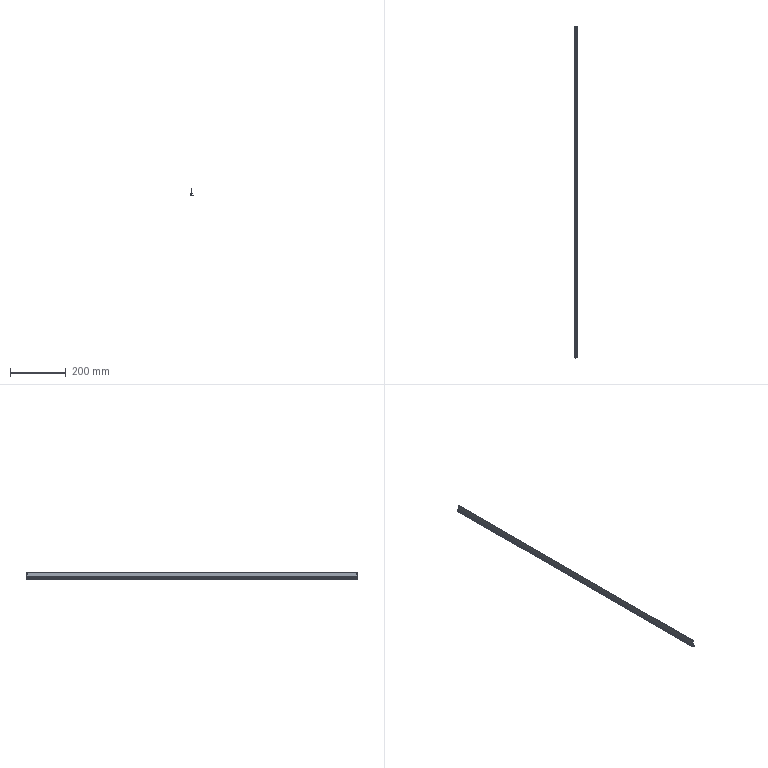Part | NX | features BREP 1 | 1 solid | 48 faces | box 8.5 x 1190 x 27 mm | volume 74453 mm3 | cylinder 25 | plane 23 | commonest cylinder face diameters 0.4 x14 1 x6 3.5 x4 2 x1